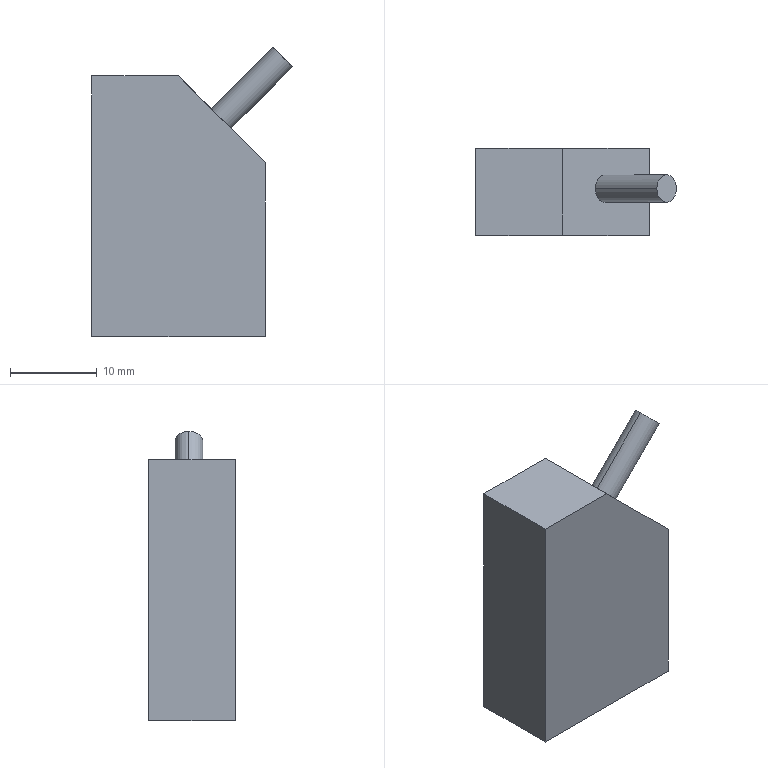Part | SolidWorks | features Chamfer 1, Extrusion 1, ICE 1 | 1 solid | 10 faces | box 23.098 x 10 x 33.285 mm | volume 5579 mm3 | plane 8 | cylinder 2 | commonest cylinder face diameters 3.169 x2
STEP:
#1=CARTESIAN_POINT('',(23.098,5.36,31.045));
#2=VERTEX_POINT('',#1);
#3=CARTESIAN_POINT('',(20.857,5.36,33.285));
#4=VERTEX_POINT('',#3);
#5=CARTESIAN_POINT('',(21.977,5.36,32.165));
#6=DIRECTION('',(0.7071,0.,0.7071));
#7=DIRECTION('',(0.7071,0.,-0.7071));
#8=AXIS2_PLACEMENT_3D('',#5,#6,#7);
#9=CIRCLE('',#8,1.584);
#10=EDGE_CURVE('',#2,#4,#9,.T.);
#11=ORIENTED_EDGE('',*,*,#10,.F.);
#12=CARTESIAN_POINT('',(16.027,5.36,23.973));
#13=VERTEX_POINT('',#12);
#14=CARTESIAN_POINT('',(23.098,5.36,31.045));
#15=DIRECTION('',(-0.7071,0.,-0.7071));
#16=VECTOR('',#15,1000.);
#17=LINE('',#14,#16);
#18=EDGE_CURVE('',#2,#13,#17,.T.);
#19=ORIENTED_EDGE('',*,*,#18,.T.);
#20=CARTESIAN_POINT('',(13.786,5.36,26.214));
#21=VERTEX_POINT('',#20);
#22=CARTESIAN_POINT('',(14.906,5.36,25.094));
#23=DIRECTION('',(0.7071,0.,0.7071));
#24=DIRECTION('',(0.7071,0.,-0.7071));
#25=AXIS2_PLACEMENT_3D('',#22,#23,#24);
#26=CIRCLE('',#25,1.584);
#27=EDGE_CURVE('',#13,#21,#26,.T.);
#28=ORIENTED_EDGE('',*,*,#27,.T.);
#29=CARTESIAN_POINT('',(20.857,5.36,33.285));
#30=DIRECTION('',(-0.7071,0.,-0.7071));
#31=VECTOR('',#30,1000.);
#32=LINE('',#29,#31);
#33=EDGE_CURVE('',#4,#21,#32,.T.);
#34=ORIENTED_EDGE('',*,*,#33,.F.);
#35=EDGE_LOOP('',(#11,#19,#28,#34));
#36=FACE_OUTER_BOUND('',#35,.T.);
#37=CARTESIAN_POINT('',(21.977,5.36,32.165));
#38=DIRECTION('',(-0.7071,0.,-0.7071));
#39=DIRECTION('',(-0.7071,0.,0.7071));
#40=AXIS2_PLACEMENT_3D('',#37,#38,#39);
#41=CYLINDRICAL_SURFACE('',#40,1.584);
#42=ADVANCED_FACE('',(#36),#41,.T.);
#43=CARTESIAN_POINT('',(0.,0.,0.));
#44=VERTEX_POINT('',#43);
#45=CARTESIAN_POINT('',(0.,0.,30.));
#46=VERTEX_POINT('',#45);
#47=CARTESIAN_POINT('',(0.,0.,0.));
#48=DIRECTION('',(0.,0.,1.));
#49=VECTOR('',#48,1000.);
#50=LINE('',#47,#49);
#51=EDGE_CURVE('',#44,#46,#50,.T.);
#52=ORIENTED_EDGE('',*,*,#51,.T.);
#53=CARTESIAN_POINT('',(0.,10.,30.));
#54=VERTEX_POINT('',#53);
#55=CARTESIAN_POINT('',(0.,10.,30.));
#56=DIRECTION('',(0.,-1.,0.));
#57=VECTOR('',#56,1000.);
#58=LINE('',#55,#57);
#59=EDGE_CURVE('',#54,#46,#58,.T.);
#60=ORIENTED_EDGE('',*,*,#59,.F.);
#61=CARTESIAN_POINT('',(0.,10.,0.));
#62=VERTEX_POINT('',#61);
#63=CARTESIAN_POINT('',(0.,10.,0.));
#64=DIRECTION('',(0.,0.,1.));
#65=VECTOR('',#64,1000.);
#66=LINE('',#63,#65);
#67=EDGE_CURVE('',#62,#54,#66,.T.);
#68=ORIENTED_EDGE('',*,*,#67,.F.);
#69=CARTESIAN_POINT('',(0.,10.,0.));
#70=DIRECTION('',(0.,-1.,0.));
#71=VECTOR('',#70,1000.);
#72=LINE('',#69,#71);
#73=EDGE_CURVE('',#62,#44,#72,.T.);
#74=ORIENTED_EDGE('',*,*,#73,.T.);
#75=EDGE_LOOP('',(#52,#60,#68,#74));
#76=FACE_OUTER_BOUND('',#75,.T.);
#77=CARTESIAN_POINT('',(0.,10.,0.));
#78=DIRECTION('',(1.,0.,0.));
#79=DIRECTION('',(0.,0.,-1.));
#80=AXIS2_PLACEMENT_3D('',#77,#78,#79);
#81=PLANE('',#80);
#82=ADVANCED_FACE('',(#76),#81,.F.);
#83=CARTESIAN_POINT('',(10.,0.,30.));
#84=VERTEX_POINT('',#83);
#85=CARTESIAN_POINT('',(0.,0.,30.));
#86=DIRECTION('',(1.,0.,0.));
#87=VECTOR('',#86,1000.);
#88=LINE('',#85,#87);
#89=EDGE_CURVE('',#46,#84,#88,.T.);
#90=ORIENTED_EDGE('',*,*,#89,.T.);
#91=CARTESIAN_POINT('',(10.,10.,30.));
#92=VERTEX_POINT('',#91);
#93=CARTESIAN_POINT('',(10.,10.,30.));
#94=DIRECTION('',(0.,1.,0.));
#95=VECTOR('',#94,1000.);
#96=LINE('',#93,#95);
#97=EDGE_CURVE('',#84,#92,#96,.T.);
#98=ORIENTED_EDGE('',*,*,#97,.T.);
#99=CARTESIAN_POINT('',(0.,10.,30.));
#100=DIRECTION('',(1.,0.,0.));
#101=VECTOR('',#100,1000.);
#102=LINE('',#99,#101);
#103=EDGE_CURVE('',#54,#92,#102,.T.);
#104=ORIENTED_EDGE('',*,*,#103,.F.);
#105=ORIENTED_EDGE('',*,*,#59,.T.);
#106=EDGE_LOOP('',(#90,#98,#104,#105));
#107=FACE_OUTER_BOUND('',#106,.T.);
#108=CARTESIAN_POINT('',(0.,10.,30.));
#109=DIRECTION('',(0.,0.,-1.));
#110=DIRECTION('',(-1.,0.,0.));
#111=AXIS2_PLACEMENT_3D('',#108,#109,#110);
#112=PLANE('',#111);
#113=ADVANCED_FACE('',(#107),#112,.F.);
#114=CARTESIAN_POINT('',(20.,10.,20.));
#115=VERTEX_POINT('',#114);
#116=CARTESIAN_POINT('',(20.,10.,0.));
#117=VERTEX_POINT('',#116);
#118=CARTESIAN_POINT('',(20.,10.,0.));
#119=DIRECTION('',(0.,0.,-1.));
#120=VECTOR('',#119,1000.);
#121=LINE('',#118,#120);
#122=EDGE_CURVE('',#115,#117,#121,.T.);
#123=ORIENTED_EDGE('',*,*,#122,.F.);
#124=CARTESIAN_POINT('',(20.,0.,20.));
#125=VERTEX_POINT('',#124);
#126=CARTESIAN_POINT('',(20.,10.,20.));
#127=DIRECTION('',(0.,-1.,0.));
#128=VECTOR('',#127,1000.);
#129=LINE('',#126,#128);
#130=EDGE_CURVE('',#115,#125,#129,.T.);
#131=ORIENTED_EDGE('',*,*,#130,.T.);
#132=CARTESIAN_POINT('',(20.,0.,0.));
#133=VERTEX_POINT('',#132);
#134=CARTESIAN_POINT('',(20.,0.,0.));
#135=DIRECTION('',(0.,0.,-1.));
#136=VECTOR('',#135,1000.);
#137=LINE('',#134,#136);
#138=EDGE_CURVE('',#125,#133,#137,.T.);
#139=ORIENTED_EDGE('',*,*,#138,.T.);
#140=CARTESIAN_POINT('',(20.,10.,0.));
#141=DIRECTION('',(0.,-1.,0.));
#142=VECTOR('',#141,1000.);
#143=LINE('',#140,#142);
#144=EDGE_CURVE('',#117,#133,#143,.T.);
#145=ORIENTED_EDGE('',*,*,#144,.F.);
#146=EDGE_LOOP('',(#123,#131,#139,#145));
#147=FACE_OUTER_BOUND('',#146,.T.);
#148=CARTESIAN_POINT('',(20.,10.,0.));
#149=DIRECTION('',(-1.,0.,0.));
#150=DIRECTION('',(0.,0.,1.));
#151=AXIS2_PLACEMENT_3D('',#148,#149,#150);
#152=PLANE('',#151);
#153=ADVANCED_FACE('',(#147),#152,.F.);
#154=CARTESIAN_POINT('',(0.,0.,0.));
#155=DIRECTION('',(-1.,0.,0.));
#156=VECTOR('',#155,1000.);
#157=LINE('',#154,#156);
#158=EDGE_CURVE('',#133,#44,#157,.T.);
#159=ORIENTED_EDGE('',*,*,#158,.T.);
#160=ORIENTED_EDGE('',*,*,#73,.F.);
#161=CARTESIAN_POINT('',(0.,10.,0.));
#162=DIRECTION('',(-1.,0.,0.));
#163=VECTOR('',#162,1000.);
#164=LINE('',#161,#163);
#165=EDGE_CURVE('',#117,#62,#164,.T.);
#166=ORIENTED_EDGE('',*,*,#165,.F.);
#167=ORIENTED_EDGE('',*,*,#144,.T.);
#168=EDGE_LOOP('',(#159,#160,#166,#167));
#169=FACE_OUTER_BOUND('',#168,.T.);
#170=CARTESIAN_POINT('',(0.,10.,0.));
#171=DIRECTION('',(0.,0.,1.));
#172=DIRECTION('',(1.,0.,0.));
#173=AXIS2_PLACEMENT_3D('',#170,#171,#172);
#174=PLANE('',#173);
#175=ADVANCED_FACE('',(#169),#174,.F.);
#176=ORIENTED_EDGE('',*,*,#103,.T.);
#177=CARTESIAN_POINT('',(20.,10.,20.));
#178=DIRECTION('',(0.7071,0.,-0.7071));
#179=VECTOR('',#178,1000.);
#180=LINE('',#177,#179);
#181=EDGE_CURVE('',#92,#115,#180,.T.);
#182=ORIENTED_EDGE('',*,*,#181,.T.);
#183=ORIENTED_EDGE('',*,*,#122,.T.);
#184=ORIENTED_EDGE('',*,*,#165,.T.);
#185=ORIENTED_EDGE('',*,*,#67,.T.);
#186=EDGE_LOOP('',(#176,#182,#183,#184,#185));
#187=FACE_OUTER_BOUND('',#186,.T.);
#188=CARTESIAN_POINT('',(0.,10.,0.));
#189=DIRECTION('',(0.,1.,0.));
#190=DIRECTION('',(0.,0.,1.));
#191=AXIS2_PLACEMENT_3D('',#188,#189,#190);
#192=PLANE('',#191);
#193=ADVANCED_FACE('',(#187),#192,.T.);
#194=ORIENTED_EDGE('',*,*,#138,.F.);
#195=CARTESIAN_POINT('',(20.,0.,20.));
#196=DIRECTION('',(-0.7071,0.,0.7071));
#197=VECTOR('',#196,1000.);
#198=LINE('',#195,#197);
#199=EDGE_CURVE('',#125,#84,#198,.T.);
#200=ORIENTED_EDGE('',*,*,#199,.T.);
#201=ORIENTED_EDGE('',*,*,#89,.F.);
#202=ORIENTED_EDGE('',*,*,#51,.F.);
#203=ORIENTED_EDGE('',*,*,#158,.F.);
#204=EDGE_LOOP('',(#194,#200,#201,#202,#203));
#205=FACE_OUTER_BOUND('',#204,.T.);
#206=CARTESIAN_POINT('',(0.,0.,0.));
#207=DIRECTION('',(0.,1.,0.));
#208=DIRECTION('',(0.,0.,1.));
#209=AXIS2_PLACEMENT_3D('',#206,#207,#208);
#210=PLANE('',#209);
#211=ADVANCED_FACE('',(#205),#210,.F.);
#212=CARTESIAN_POINT('',(14.906,5.36,25.094));
#213=DIRECTION('',(0.7071,0.,0.7071));
#214=DIRECTION('',(0.7071,0.,-0.7071));
#215=AXIS2_PLACEMENT_3D('',#212,#213,#214);
#216=CIRCLE('',#215,1.584);
#217=EDGE_CURVE('',#21,#13,#216,.T.);
#218=ORIENTED_EDGE('',*,*,#217,.F.);
#219=ORIENTED_EDGE('',*,*,#27,.F.);
#220=EDGE_LOOP('',(#218,#219));
#221=FACE_BOUND('',#220,.T.);
#222=ORIENTED_EDGE('',*,*,#181,.F.);
#223=ORIENTED_EDGE('',*,*,#97,.F.);
#224=ORIENTED_EDGE('',*,*,#199,.F.);
#225=ORIENTED_EDGE('',*,*,#130,.F.);
#226=EDGE_LOOP('',(#222,#223,#224,#225));
#227=FACE_OUTER_BOUND('',#226,.T.);
#228=CARTESIAN_POINT('',(20.,10.,20.));
#229=DIRECTION('',(-0.7071,0.,-0.7071));
#230=DIRECTION('',(0.,-1.,0.));
#231=AXIS2_PLACEMENT_3D('',#228,#229,#230);
#232=PLANE('',#231);
#233=ADVANCED_FACE('',(#221,#227),#232,.F.);
#234=ORIENTED_EDGE('',*,*,#18,.F.);
#235=CARTESIAN_POINT('',(21.977,5.36,32.165));
#236=DIRECTION('',(0.7071,0.,0.7071));
#237=DIRECTION('',(0.7071,0.,-0.7071));
#238=AXIS2_PLACEMENT_3D('',#235,#236,#237);
#239=CIRCLE('',#238,1.584);
#240=EDGE_CURVE('',#4,#2,#239,.T.);
#241=ORIENTED_EDGE('',*,*,#240,.F.);
#242=ORIENTED_EDGE('',*,*,#33,.T.);
#243=ORIENTED_EDGE('',*,*,#217,.T.);
#244=EDGE_LOOP('',(#234,#241,#242,#243));
#245=FACE_OUTER_BOUND('',#244,.T.);
#246=CARTESIAN_POINT('',(21.977,5.36,32.165));
#247=DIRECTION('',(-0.7071,0.,-0.7071));
#248=DIRECTION('',(-0.7071,0.,0.7071));
#249=AXIS2_PLACEMENT_3D('',#246,#247,#248);
#250=CYLINDRICAL_SURFACE('',#249,1.584);
#251=ADVANCED_FACE('',(#245),#250,.T.);
#252=ORIENTED_EDGE('',*,*,#240,.T.);
#253=ORIENTED_EDGE('',*,*,#10,.T.);
#254=EDGE_LOOP('',(#252,#253));
#255=FACE_OUTER_BOUND('',#254,.T.);
#256=CARTESIAN_POINT('',(21.977,5.36,32.165));
#257=DIRECTION('',(0.7071,0.,0.7071));
#258=DIRECTION('',(0.7071,0.,-0.7071));
#259=AXIS2_PLACEMENT_3D('',#256,#257,#258);
#260=PLANE('',#259);
#261=ADVANCED_FACE('',(#255),#260,.T.);
#262=CLOSED_SHELL('',(#42,#82,#113,#153,#175,#193,#211,#233,#251,#261));
#263=MANIFOLD_SOLID_BREP('',#262);
#264=CARTESIAN_POINT('',(0.,0.,0.));
#265=DIRECTION('',(0.,0.,1.));
#266=DIRECTION('',(1.,0.,0.));
#267=AXIS2_PLACEMENT_3D('',#264,#265,#266);
#268=(LENGTH_UNIT()NAMED_UNIT(*)SI_UNIT(.MILLI.,.METRE.));
#269=UNCERTAINTY_MEASURE_WITH_UNIT(LENGTH_MEASURE(0.00001),#268,'','');
#270=(NAMED_UNIT(*)PLANE_ANGLE_UNIT()SI_UNIT($,.RADIAN.));
#271=(NAMED_UNIT(*)SI_UNIT($,.STERADIAN.)SOLID_ANGLE_UNIT());
#272=(GEOMETRIC_REPRESENTATION_CONTEXT(3)GLOBAL_UNCERTAINTY_ASSIGNED_CONTEXT((#269))GLOBAL_UNIT_ASSIGNED_CONTEXT((#268,#270,#271))REPRESENTATION_CONTEXT('',''));
#273=ADVANCED_BREP_SHAPE_REPRESENTATION('',(#263,#267),#272);